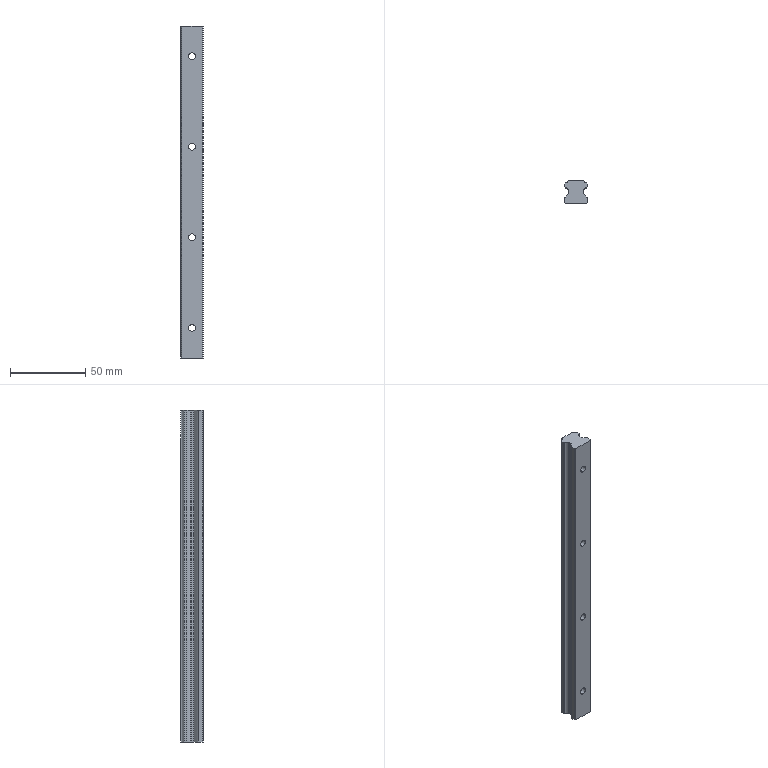Part | STEP file | HGR15_1 | 1 solid | 56 faces | box 15 x 15 x 220 mm | volume 40412 mm3 | cylinder 30 | plane 26 | commonest cylinder face diameters 0.8 x8 4.5 x8 7.5 x6 3.24 x4 2 x2 8 x2